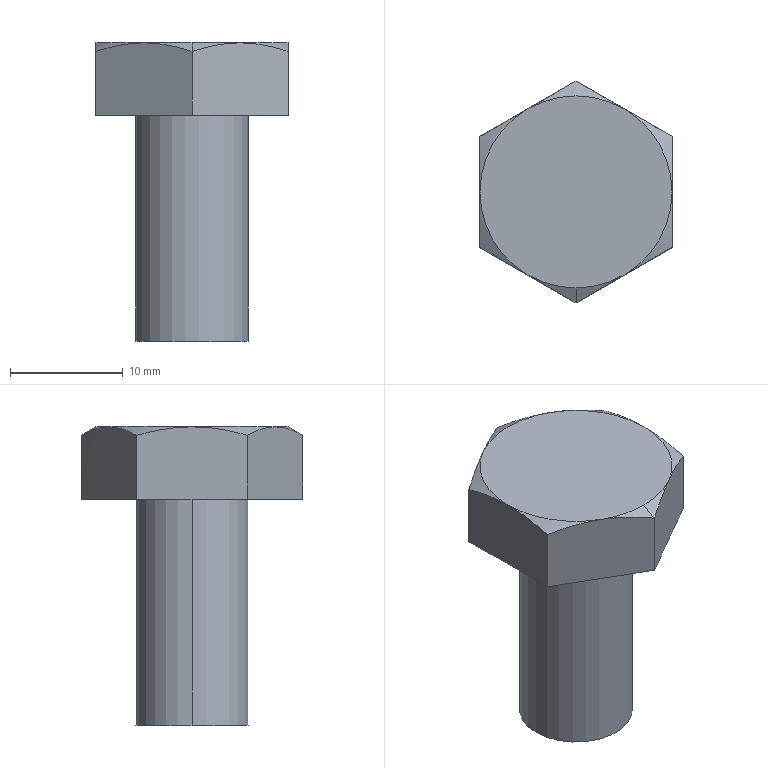Part | SolidWorks | features ICE 1, MBimport 1 | 1 solid | 18 faces | box 17 x 19.63 x 26.4 mm | volume 3167 mm3 | plane 9 | cone 7 | cylinder 2 | commonest cylinder face diameters 10 x2
STEP:
#1=CARTESIAN_POINT('',(-5.,0.,-10.));
#2=VERTEX_POINT('',#1);
#3=CARTESIAN_POINT('',(5.,0.,-10.));
#4=VERTEX_POINT('',#3);
#5=CARTESIAN_POINT('',(0.,0.,-10.));
#6=DIRECTION('',(0.,0.,-1.));
#7=DIRECTION('',(-1.,0.,0.));
#8=AXIS2_PLACEMENT_3D('',#5,#6,#7);
#9=CIRCLE('',#8,5.);
#10=EDGE_CURVE('',#2,#4,#9,.T.);
#11=ORIENTED_EDGE('',*,*,#10,.F.);
#12=CARTESIAN_POINT('',(-5.,0.,10.));
#13=VERTEX_POINT('',#12);
#14=CARTESIAN_POINT('',(-5.,0.,0.));
#15=DIRECTION('',(0.,0.,1.));
#16=VECTOR('',#15,1000.);
#17=LINE('',#14,#16);
#18=EDGE_CURVE('',#2,#13,#17,.T.);
#19=ORIENTED_EDGE('',*,*,#18,.T.);
#20=CARTESIAN_POINT('',(5.,0.,10.));
#21=VERTEX_POINT('',#20);
#22=CARTESIAN_POINT('',(0.,0.,10.));
#23=DIRECTION('',(0.,0.,1.));
#24=DIRECTION('',(-1.,0.,0.));
#25=AXIS2_PLACEMENT_3D('',#22,#23,#24);
#26=CIRCLE('',#25,5.);
#27=EDGE_CURVE('',#21,#13,#26,.T.);
#28=ORIENTED_EDGE('',*,*,#27,.F.);
#29=CARTESIAN_POINT('',(5.,0.,0.));
#30=DIRECTION('',(0.,0.,1.));
#31=VECTOR('',#30,1000.);
#32=LINE('',#29,#31);
#33=EDGE_CURVE('',#4,#21,#32,.T.);
#34=ORIENTED_EDGE('',*,*,#33,.F.);
#35=EDGE_LOOP('',(#11,#19,#28,#34));
#36=FACE_OUTER_BOUND('',#35,.T.);
#37=CARTESIAN_POINT('',(0.,0.,0.));
#38=DIRECTION('',(0.,0.,1.));
#39=DIRECTION('',(1.,0.,0.));
#40=AXIS2_PLACEMENT_3D('',#37,#38,#39);
#41=CYLINDRICAL_SURFACE('',#40,5.);
#42=ADVANCED_FACE('',(#36),#41,.T.);
#43=CARTESIAN_POINT('',(0.,-8.5,16.4));
#44=VERTEX_POINT('',#43);
#45=CARTESIAN_POINT('',(4.25,-7.361,16.4));
#46=VERTEX_POINT('',#45);
#47=CARTESIAN_POINT('',(0.,0.,16.4));
#48=DIRECTION('',(0.,0.,1.));
#49=DIRECTION('',(-0.5,-0.866,0.));
#50=AXIS2_PLACEMENT_3D('',#47,#48,#49);
#51=CIRCLE('',#50,8.5);
#52=EDGE_CURVE('',#44,#46,#51,.T.);
#53=ORIENTED_EDGE('',*,*,#52,.F.);
#54=CARTESIAN_POINT('',(0.,-9.815,15.641));
#55=VERTEX_POINT('',#54);
#56=CARTESIAN_POINT('',(0.,-9.157,16.02));
#57=DIRECTION('',(0.,-0.866,-0.5));
#58=VECTOR('',#57,1000.);
#59=LINE('',#56,#58);
#60=EDGE_CURVE('',#44,#55,#59,.T.);
#61=ORIENTED_EDGE('',*,*,#60,.T.);
#62=CARTESIAN_POINT('',(0.,-9.815,15.641));
#63=CARTESIAN_POINT('',(0.3728,-9.6,15.765));
#64=CARTESIAN_POINT('',(0.7368,-9.389,15.874));
#65=CARTESIAN_POINT('',(1.275,-9.078,16.016));
#66=CARTESIAN_POINT('',(1.454,-8.975,16.059));
#67=CARTESIAN_POINT('',(1.809,-8.771,16.138));
#68=CARTESIAN_POINT('',(1.987,-8.668,16.175));
#69=CARTESIAN_POINT('',(2.514,-8.364,16.27));
#70=CARTESIAN_POINT('',(2.858,-8.165,16.318));
#71=CARTESIAN_POINT('',(3.557,-7.762,16.384));
#72=CARTESIAN_POINT('',(3.902,-7.562,16.4));
#73=CARTESIAN_POINT('',(4.25,-7.361,16.4));
#74=B_SPLINE_CURVE_WITH_KNOTS('',3,(#62,#63,#64,#65,#66,#67,#68,#69,#70,#71,#72,#73),.UNSPECIFIED.,.F.,.F.,(4,2,2,2,2,4),(0.,0.25,0.375,0.5,0.75,1.),.UNSPECIFIED.);
#75=EDGE_CURVE('',#55,#46,#74,.T.);
#76=ORIENTED_EDGE('',*,*,#75,.T.);
#77=EDGE_LOOP('',(#53,#61,#76));
#78=FACE_OUTER_BOUND('',#77,.T.);
#79=CARTESIAN_POINT('',(0.,0.,16.02));
#80=DIRECTION('',(0.,0.,-1.));
#81=DIRECTION('',(0.,-1.,0.));
#82=AXIS2_PLACEMENT_3D('',#79,#80,#81);
#83=CONICAL_SURFACE('',#82,9.157,1.047);
#84=ADVANCED_FACE('',(#78),#83,.T.);
#85=CARTESIAN_POINT('',(-8.5,4.907,10.));
#86=VERTEX_POINT('',#85);
#87=CARTESIAN_POINT('',(-8.5,4.907,15.641));
#88=VERTEX_POINT('',#87);
#89=CARTESIAN_POINT('',(-8.5,4.907,10.));
#90=DIRECTION('',(0.,0.,1.));
#91=VECTOR('',#90,1000.);
#92=LINE('',#89,#91);
#93=EDGE_CURVE('',#86,#88,#92,.T.);
#94=ORIENTED_EDGE('',*,*,#93,.F.);
#95=CARTESIAN_POINT('',(-8.5,-4.907,10.));
#96=VERTEX_POINT('',#95);
#97=CARTESIAN_POINT('',(-8.5,4.907,10.));
#98=DIRECTION('',(0.,-1.,0.));
#99=VECTOR('',#98,1000.);
#100=LINE('',#97,#99);
#101=EDGE_CURVE('',#86,#96,#100,.T.);
#102=ORIENTED_EDGE('',*,*,#101,.T.);
#103=CARTESIAN_POINT('',(-8.5,-4.907,15.641));
#104=VERTEX_POINT('',#103);
#105=CARTESIAN_POINT('',(-8.5,-4.907,10.));
#106=DIRECTION('',(0.,0.,1.));
#107=VECTOR('',#106,1000.);
#108=LINE('',#105,#107);
#109=EDGE_CURVE('',#96,#104,#108,.T.);
#110=ORIENTED_EDGE('',*,*,#109,.T.);
#111=CARTESIAN_POINT('',(-8.5,0.,16.4));
#112=VERTEX_POINT('',#111);
#113=CARTESIAN_POINT('',(-8.5,0.,16.4));
#114=CARTESIAN_POINT('',(-8.5,-0.201,16.4));
#115=CARTESIAN_POINT('',(-8.5,-0.4012,16.396));
#116=CARTESIAN_POINT('',(-8.5,-0.8019,16.38));
#117=CARTESIAN_POINT('',(-8.5,-1.004,16.367));
#118=CARTESIAN_POINT('',(-8.5,-1.405,16.335));
#119=CARTESIAN_POINT('',(-8.5,-1.605,16.315));
#120=CARTESIAN_POINT('',(-8.5,-2.007,16.266));
#121=CARTESIAN_POINT('',(-8.5,-2.207,16.239));
#122=CARTESIAN_POINT('',(-8.5,-3.227,16.078));
#123=CARTESIAN_POINT('',(-8.5,-4.047,15.889));
#124=CARTESIAN_POINT('',(-8.5,-4.907,15.641));
#125=B_SPLINE_CURVE_WITH_KNOTS('',3,(#113,#114,#115,#116,#117,#118,#119,#120,#121,#122,#123,#124),.UNSPECIFIED.,.F.,.F.,(4,2,2,2,2,4),(0.,0.125,0.25,0.375,0.5,1.),.UNSPECIFIED.);
#126=EDGE_CURVE('',#112,#104,#125,.T.);
#127=ORIENTED_EDGE('',*,*,#126,.F.);
#128=CARTESIAN_POINT('',(-8.5,4.907,15.641));
#129=CARTESIAN_POINT('',(-8.5,4.477,15.765));
#130=CARTESIAN_POINT('',(-8.5,4.057,15.874));
#131=CARTESIAN_POINT('',(-8.5,3.435,16.016));
#132=CARTESIAN_POINT('',(-8.5,3.229,16.059));
#133=CARTESIAN_POINT('',(-8.5,2.819,16.138));
#134=CARTESIAN_POINT('',(-8.5,2.613,16.175));
#135=CARTESIAN_POINT('',(-8.5,2.005,16.27));
#136=CARTESIAN_POINT('',(-8.5,1.607,16.318));
#137=CARTESIAN_POINT('',(-8.5,0.8006,16.384));
#138=CARTESIAN_POINT('',(-8.5,0.402,16.4));
#139=CARTESIAN_POINT('',(-8.5,0.,16.4));
#140=B_SPLINE_CURVE_WITH_KNOTS('',3,(#128,#129,#130,#131,#132,#133,#134,#135,#136,#137,#138,#139),.UNSPECIFIED.,.F.,.F.,(4,2,2,2,2,4),(0.,0.25,0.375,0.5,0.75,1.),.UNSPECIFIED.);
#141=EDGE_CURVE('',#88,#112,#140,.T.);
#142=ORIENTED_EDGE('',*,*,#141,.F.);
#143=EDGE_LOOP('',(#94,#102,#110,#127,#142));
#144=FACE_OUTER_BOUND('',#143,.T.);
#145=CARTESIAN_POINT('',(-8.5,4.907,10.));
#146=DIRECTION('',(-1.,0.,0.));
#147=DIRECTION('',(0.,0.,1.));
#148=AXIS2_PLACEMENT_3D('',#145,#146,#147);
#149=PLANE('',#148);
#150=ADVANCED_FACE('',(#144),#149,.T.);
#151=ORIENTED_EDGE('',*,*,#109,.F.);
#152=CARTESIAN_POINT('',(0.,-9.815,10.));
#153=VERTEX_POINT('',#152);
#154=CARTESIAN_POINT('',(-8.5,-4.907,10.));
#155=DIRECTION('',(0.866,-0.5,0.));
#156=VECTOR('',#155,1000.);
#157=LINE('',#154,#156);
#158=EDGE_CURVE('',#96,#153,#157,.T.);
#159=ORIENTED_EDGE('',*,*,#158,.T.);
#160=CARTESIAN_POINT('',(0.,-9.815,10.));
#161=DIRECTION('',(0.,0.,1.));
#162=VECTOR('',#161,1000.);
#163=LINE('',#160,#162);
#164=EDGE_CURVE('',#153,#55,#163,.T.);
#165=ORIENTED_EDGE('',*,*,#164,.T.);
#166=CARTESIAN_POINT('',(-4.25,-7.361,16.4));
#167=VERTEX_POINT('',#166);
#168=CARTESIAN_POINT('',(-4.25,-7.361,16.4));
#169=CARTESIAN_POINT('',(-4.076,-7.462,16.4));
#170=CARTESIAN_POINT('',(-3.903,-7.562,16.396));
#171=CARTESIAN_POINT('',(-3.556,-7.762,16.38));
#172=CARTESIAN_POINT('',(-3.381,-7.863,16.367));
#173=CARTESIAN_POINT('',(-3.034,-8.064,16.335));
#174=CARTESIAN_POINT('',(-2.86,-8.164,16.315));
#175=CARTESIAN_POINT('',(-2.512,-8.365,16.266));
#176=CARTESIAN_POINT('',(-2.339,-8.465,16.239));
#177=CARTESIAN_POINT('',(-1.455,-8.975,16.078));
#178=CARTESIAN_POINT('',(-0.7455,-9.385,15.889));
#179=CARTESIAN_POINT('',(0.,-9.815,15.641));
#180=B_SPLINE_CURVE_WITH_KNOTS('',3,(#168,#169,#170,#171,#172,#173,#174,#175,#176,#177,#178,#179),.UNSPECIFIED.,.F.,.F.,(4,2,2,2,2,4),(0.,0.125,0.25,0.375,0.5,1.),.UNSPECIFIED.);
#181=EDGE_CURVE('',#167,#55,#180,.T.);
#182=ORIENTED_EDGE('',*,*,#181,.F.);
#183=CARTESIAN_POINT('',(-8.5,-4.907,15.641));
#184=CARTESIAN_POINT('',(-8.127,-5.123,15.765));
#185=CARTESIAN_POINT('',(-7.763,-5.333,15.874));
#186=CARTESIAN_POINT('',(-7.224,-5.644,16.016));
#187=CARTESIAN_POINT('',(-7.046,-5.747,16.059));
#188=CARTESIAN_POINT('',(-6.691,-5.952,16.138));
#189=CARTESIAN_POINT('',(-6.513,-6.054,16.175));
#190=CARTESIAN_POINT('',(-5.986,-6.359,16.27));
#191=CARTESIAN_POINT('',(-5.642,-6.558,16.318));
#192=CARTESIAN_POINT('',(-4.943,-6.961,16.384));
#193=CARTESIAN_POINT('',(-4.598,-7.16,16.4));
#194=CARTESIAN_POINT('',(-4.25,-7.361,16.4));
#195=B_SPLINE_CURVE_WITH_KNOTS('',3,(#183,#184,#185,#186,#187,#188,#189,#190,#191,#192,#193,#194),.UNSPECIFIED.,.F.,.F.,(4,2,2,2,2,4),(0.,0.25,0.375,0.5,0.75,1.),.UNSPECIFIED.);
#196=EDGE_CURVE('',#104,#167,#195,.T.);
#197=ORIENTED_EDGE('',*,*,#196,.F.);
#198=EDGE_LOOP('',(#151,#159,#165,#182,#197));
#199=FACE_OUTER_BOUND('',#198,.T.);
#200=CARTESIAN_POINT('',(-8.5,-4.907,10.));
#201=DIRECTION('',(-0.5,-0.866,0.));
#202=DIRECTION('',(-0.866,0.5,0.));
#203=AXIS2_PLACEMENT_3D('',#200,#201,#202);
#204=PLANE('',#203);
#205=ADVANCED_FACE('',(#199),#204,.T.);
#206=ORIENTED_EDGE('',*,*,#164,.F.);
#207=CARTESIAN_POINT('',(8.5,-4.907,10.));
#208=VERTEX_POINT('',#207);
#209=CARTESIAN_POINT('',(0.,-9.815,10.));
#210=DIRECTION('',(0.866,0.5,0.));
#211=VECTOR('',#210,1000.);
#212=LINE('',#209,#211);
#213=EDGE_CURVE('',#153,#208,#212,.T.);
#214=ORIENTED_EDGE('',*,*,#213,.T.);
#215=CARTESIAN_POINT('',(8.5,-4.907,15.641));
#216=VERTEX_POINT('',#215);
#217=CARTESIAN_POINT('',(8.5,-4.907,10.));
#218=DIRECTION('',(0.,0.,1.));
#219=VECTOR('',#218,1000.);
#220=LINE('',#217,#219);
#221=EDGE_CURVE('',#208,#216,#220,.T.);
#222=ORIENTED_EDGE('',*,*,#221,.T.);
#223=CARTESIAN_POINT('',(4.25,-7.361,16.4));
#224=CARTESIAN_POINT('',(4.424,-7.261,16.4));
#225=CARTESIAN_POINT('',(4.597,-7.161,16.396));
#226=CARTESIAN_POINT('',(4.944,-6.96,16.38));
#227=CARTESIAN_POINT('',(5.119,-6.859,16.367));
#228=CARTESIAN_POINT('',(5.466,-6.659,16.335));
#229=CARTESIAN_POINT('',(5.64,-6.559,16.315));
#230=CARTESIAN_POINT('',(5.988,-6.358,16.266));
#231=CARTESIAN_POINT('',(6.161,-6.258,16.239));
#232=CARTESIAN_POINT('',(7.045,-5.748,16.078));
#233=CARTESIAN_POINT('',(7.754,-5.338,15.889));
#234=CARTESIAN_POINT('',(8.5,-4.907,15.641));
#235=B_SPLINE_CURVE_WITH_KNOTS('',3,(#223,#224,#225,#226,#227,#228,#229,#230,#231,#232,#233,#234),.UNSPECIFIED.,.F.,.F.,(4,2,2,2,2,4),(0.,0.125,0.25,0.375,0.5,1.),.UNSPECIFIED.);
#236=EDGE_CURVE('',#46,#216,#235,.T.);
#237=ORIENTED_EDGE('',*,*,#236,.F.);
#238=ORIENTED_EDGE('',*,*,#75,.F.);
#239=EDGE_LOOP('',(#206,#214,#222,#237,#238));
#240=FACE_OUTER_BOUND('',#239,.T.);
#241=CARTESIAN_POINT('',(0.,-9.815,10.));
#242=DIRECTION('',(0.5,-0.866,0.));
#243=DIRECTION('',(0.,0.,-1.));
#244=AXIS2_PLACEMENT_3D('',#241,#242,#243);
#245=PLANE('',#244);
#246=ADVANCED_FACE('',(#240),#245,.T.);
#247=ORIENTED_EDGE('',*,*,#221,.F.);
#248=CARTESIAN_POINT('',(8.5,4.907,10.));
#249=VERTEX_POINT('',#248);
#250=CARTESIAN_POINT('',(8.5,-4.907,10.));
#251=DIRECTION('',(0.,1.,0.));
#252=VECTOR('',#251,1000.);
#253=LINE('',#250,#252);
#254=EDGE_CURVE('',#208,#249,#253,.T.);
#255=ORIENTED_EDGE('',*,*,#254,.T.);
#256=CARTESIAN_POINT('',(8.5,4.907,15.641));
#257=VERTEX_POINT('',#256);
#258=CARTESIAN_POINT('',(8.5,4.907,10.));
#259=DIRECTION('',(0.,0.,1.));
#260=VECTOR('',#259,1000.);
#261=LINE('',#258,#260);
#262=EDGE_CURVE('',#249,#257,#261,.T.);
#263=ORIENTED_EDGE('',*,*,#262,.T.);
#264=CARTESIAN_POINT('',(8.5,0.,16.4));
#265=VERTEX_POINT('',#264);
#266=CARTESIAN_POINT('',(8.5,0.,16.4));
#267=CARTESIAN_POINT('',(8.5,0.201,16.4));
#268=CARTESIAN_POINT('',(8.5,0.4012,16.396));
#269=CARTESIAN_POINT('',(8.5,0.8019,16.38));
#270=CARTESIAN_POINT('',(8.5,1.004,16.367));
#271=CARTESIAN_POINT('',(8.5,1.405,16.335));
#272=CARTESIAN_POINT('',(8.5,1.605,16.315));
#273=CARTESIAN_POINT('',(8.5,2.007,16.266));
#274=CARTESIAN_POINT('',(8.5,2.207,16.239));
#275=CARTESIAN_POINT('',(8.5,3.227,16.078));
#276=CARTESIAN_POINT('',(8.5,4.047,15.889));
#277=CARTESIAN_POINT('',(8.5,4.907,15.641));
#278=B_SPLINE_CURVE_WITH_KNOTS('',3,(#266,#267,#268,#269,#270,#271,#272,#273,#274,#275,#276,#277),.UNSPECIFIED.,.F.,.F.,(4,2,2,2,2,4),(0.,0.125,0.25,0.375,0.5,1.),.UNSPECIFIED.);
#279=EDGE_CURVE('',#265,#257,#278,.T.);
#280=ORIENTED_EDGE('',*,*,#279,.F.);
#281=CARTESIAN_POINT('',(8.5,-4.907,15.641));
#282=CARTESIAN_POINT('',(8.5,-4.477,15.765));
#283=CARTESIAN_POINT('',(8.5,-4.057,15.874));
#284=CARTESIAN_POINT('',(8.5,-3.435,16.016));
#285=CARTESIAN_POINT('',(8.5,-3.229,16.059));
#286=CARTESIAN_POINT('',(8.5,-2.819,16.138));
#287=CARTESIAN_POINT('',(8.5,-2.613,16.175));
#288=CARTESIAN_POINT('',(8.5,-2.005,16.27));
#289=CARTESIAN_POINT('',(8.5,-1.607,16.318));
#290=CARTESIAN_POINT('',(8.5,-0.8006,16.384));
#291=CARTESIAN_POINT('',(8.5,-0.402,16.4));
#292=CARTESIAN_POINT('',(8.5,0.,16.4));
#293=B_SPLINE_CURVE_WITH_KNOTS('',3,(#281,#282,#283,#284,#285,#286,#287,#288,#289,#290,#291,#292),.UNSPECIFIED.,.F.,.F.,(4,2,2,2,2,4),(0.,0.25,0.375,0.5,0.75,1.),.UNSPECIFIED.);
#294=EDGE_CURVE('',#216,#265,#293,.T.);
#295=ORIENTED_EDGE('',*,*,#294,.F.);
#296=EDGE_LOOP('',(#247,#255,#263,#280,#295));
#297=FACE_OUTER_BOUND('',#296,.T.);
#298=CARTESIAN_POINT('',(8.5,-4.907,10.));
#299=DIRECTION('',(1.,0.,0.));
#300=DIRECTION('',(0.,1.,0.));
#301=AXIS2_PLACEMENT_3D('',#298,#299,#300);
#302=PLANE('',#301);
#303=ADVANCED_FACE('',(#297),#302,.T.);
#304=ORIENTED_EDGE('',*,*,#262,.F.);
#305=CARTESIAN_POINT('',(0.,9.815,10.));
#306=VERTEX_POINT('',#305);
#307=CARTESIAN_POINT('',(8.5,4.907,10.));
#308=DIRECTION('',(-0.866,0.5,0.));
#309=VECTOR('',#308,1000.);
#310=LINE('',#307,#309);
#311=EDGE_CURVE('',#249,#306,#310,.T.);
#312=ORIENTED_EDGE('',*,*,#311,.T.);
#313=CARTESIAN_POINT('',(0.,9.815,15.641));
#314=VERTEX_POINT('',#313);
#315=CARTESIAN_POINT('',(0.,9.815,10.));
#316=DIRECTION('',(0.,0.,1.));
#317=VECTOR('',#316,1000.);
#318=LINE('',#315,#317);
#319=EDGE_CURVE('',#306,#314,#318,.T.);
#320=ORIENTED_EDGE('',*,*,#319,.T.);
#321=CARTESIAN_POINT('',(4.25,7.361,16.4));
#322=VERTEX_POINT('',#321);
#323=CARTESIAN_POINT('',(4.25,7.361,16.4));
#324=CARTESIAN_POINT('',(4.076,7.462,16.4));
#325=CARTESIAN_POINT('',(3.903,7.562,16.396));
#326=CARTESIAN_POINT('',(3.556,7.762,16.38));
#327=CARTESIAN_POINT('',(3.381,7.863,16.367));
#328=CARTESIAN_POINT('',(3.034,8.064,16.335));
#329=CARTESIAN_POINT('',(2.86,8.164,16.315));
#330=CARTESIAN_POINT('',(2.512,8.365,16.266));
#331=CARTESIAN_POINT('',(2.339,8.465,16.239));
#332=CARTESIAN_POINT('',(1.455,8.975,16.078));
#333=CARTESIAN_POINT('',(0.7455,9.385,15.889));
#334=CARTESIAN_POINT('',(0.,9.815,15.641));
#335=B_SPLINE_CURVE_WITH_KNOTS('',3,(#323,#324,#325,#326,#327,#328,#329,#330,#331,#332,#333,#334),.UNSPECIFIED.,.F.,.F.,(4,2,2,2,2,4),(0.,0.125,0.25,0.375,0.5,1.),.UNSPECIFIED.);
#336=EDGE_CURVE('',#322,#314,#335,.T.);
#337=ORIENTED_EDGE('',*,*,#336,.F.);
#338=CARTESIAN_POINT('',(8.5,4.907,15.641));
#339=CARTESIAN_POINT('',(8.127,5.123,15.765));
#340=CARTESIAN_POINT('',(7.763,5.333,15.874));
#341=CARTESIAN_POINT('',(7.224,5.644,16.016));
#342=CARTESIAN_POINT('',(7.046,5.747,16.059));
#343=CARTESIAN_POINT('',(6.691,5.952,16.138));
#344=CARTESIAN_POINT('',(6.513,6.054,16.175));
#345=CARTESIAN_POINT('',(5.986,6.359,16.27));
#346=CARTESIAN_POINT('',(5.642,6.558,16.318));
#347=CARTESIAN_POINT('',(4.943,6.961,16.384));
#348=CARTESIAN_POINT('',(4.598,7.16,16.4));
#349=CARTESIAN_POINT('',(4.25,7.361,16.4));
#350=B_SPLINE_CURVE_WITH_KNOTS('',3,(#338,#339,#340,#341,#342,#343,#344,#345,#346,#347,#348,#349),.UNSPECIFIED.,.F.,.F.,(4,2,2,2,2,4),(0.,0.25,0.375,0.5,0.75,1.),.UNSPECIFIED.);
#351=EDGE_CURVE('',#257,#322,#350,.T.);
#352=ORIENTED_EDGE('',*,*,#351,.F.);
#353=EDGE_LOOP('',(#304,#312,#320,#337,#352));
#354=FACE_OUTER_BOUND('',#353,.T.);
#355=CARTESIAN_POINT('',(8.5,4.907,10.));
#356=DIRECTION('',(0.5,0.866,0.));
#357=DIRECTION('',(0.,0.,-1.));
#358=AXIS2_PLACEMENT_3D('',#355,#356,#357);
#359=PLANE('',#358);
#360=ADVANCED_FACE('',(#354),#359,.T.);
#361=ORIENTED_EDGE('',*,*,#60,.F.);
#362=CARTESIAN_POINT('',(0.,0.,16.4));
#363=DIRECTION('',(0.,0.,1.));
#364=DIRECTION('',(-0.5,-0.866,0.));
#365=AXIS2_PLACEMENT_3D('',#362,#363,#364);
#366=CIRCLE('',#365,8.5);
#367=EDGE_CURVE('',#167,#44,#366,.T.);
#368=ORIENTED_EDGE('',*,*,#367,.F.);
#369=ORIENTED_EDGE('',*,*,#181,.T.);
#370=EDGE_LOOP('',(#361,#368,#369));
#371=FACE_OUTER_BOUND('',#370,.T.);
#372=CARTESIAN_POINT('',(0.,0.,16.02));
#373=DIRECTION('',(0.,0.,-1.));
#374=DIRECTION('',(0.,-1.,0.));
#375=AXIS2_PLACEMENT_3D('',#372,#373,#374);
#376=CONICAL_SURFACE('',#375,9.157,1.047);
#377=ADVANCED_FACE('',(#371),#376,.T.);
#378=ORIENTED_EDGE('',*,*,#126,.T.);
#379=ORIENTED_EDGE('',*,*,#196,.T.);
#380=CARTESIAN_POINT('',(0.,0.,16.4));
#381=DIRECTION('',(0.,0.,1.));
#382=DIRECTION('',(-1.,0.,0.));
#383=AXIS2_PLACEMENT_3D('',#380,#381,#382);
#384=CIRCLE('',#383,8.5);
#385=EDGE_CURVE('',#112,#167,#384,.T.);
#386=ORIENTED_EDGE('',*,*,#385,.F.);
#387=EDGE_LOOP('',(#378,#379,#386));
#388=FACE_OUTER_BOUND('',#387,.T.);
#389=CARTESIAN_POINT('',(0.,0.,16.02));
#390=DIRECTION('',(0.,0.,-1.));
#391=DIRECTION('',(0.,-1.,0.));
#392=AXIS2_PLACEMENT_3D('',#389,#390,#391);
#393=CONICAL_SURFACE('',#392,9.157,1.047);
#394=ADVANCED_FACE('',(#388),#393,.T.);
#395=CARTESIAN_POINT('',(-4.25,7.361,16.4));
#396=VERTEX_POINT('',#395);
#397=CARTESIAN_POINT('',(-4.25,7.361,16.4));
#398=CARTESIAN_POINT('',(-4.424,7.261,16.4));
#399=CARTESIAN_POINT('',(-4.597,7.161,16.396));
#400=CARTESIAN_POINT('',(-4.944,6.96,16.38));
#401=CARTESIAN_POINT('',(-5.119,6.859,16.367));
#402=CARTESIAN_POINT('',(-5.466,6.659,16.335));
#403=CARTESIAN_POINT('',(-5.64,6.559,16.315));
#404=CARTESIAN_POINT('',(-5.988,6.358,16.266));
#405=CARTESIAN_POINT('',(-6.161,6.258,16.239));
#406=CARTESIAN_POINT('',(-7.045,5.748,16.078));
#407=CARTESIAN_POINT('',(-7.754,5.338,15.889));
#408=CARTESIAN_POINT('',(-8.5,4.907,15.641));
#409=B_SPLINE_CURVE_WITH_KNOTS('',3,(#397,#398,#399,#400,#401,#402,#403,#404,#405,#406,#407,#408),.UNSPECIFIED.,.F.,.F.,(4,2,2,2,2,4),(0.,0.125,0.25,0.375,0.5,1.),.UNSPECIFIED.);
#410=EDGE_CURVE('',#396,#88,#409,.T.);
#411=ORIENTED_EDGE('',*,*,#410,.T.);
#412=ORIENTED_EDGE('',*,*,#141,.T.);
#413=CARTESIAN_POINT('',(0.,0.,16.4));
#414=DIRECTION('',(0.,0.,1.));
#415=DIRECTION('',(-0.5,0.866,0.));
#416=AXIS2_PLACEMENT_3D('',#413,#414,#415);
#417=CIRCLE('',#416,8.5);
#418=EDGE_CURVE('',#396,#112,#417,.T.);
#419=ORIENTED_EDGE('',*,*,#418,.F.);
#420=EDGE_LOOP('',(#411,#412,#419));
#421=FACE_OUTER_BOUND('',#420,.T.);
#422=CARTESIAN_POINT('',(0.,0.,16.02));
#423=DIRECTION('',(0.,0.,-1.));
#424=DIRECTION('',(0.,-1.,0.));
#425=AXIS2_PLACEMENT_3D('',#422,#423,#424);
#426=CONICAL_SURFACE('',#425,9.157,1.047);
#427=ADVANCED_FACE('',(#421),#426,.T.);
#428=ORIENTED_EDGE('',*,*,#236,.T.);
#429=ORIENTED_EDGE('',*,*,#294,.T.);
#430=CARTESIAN_POINT('',(0.,0.,16.4));
#431=DIRECTION('',(0.,0.,1.));
#432=DIRECTION('',(0.5,-0.866,0.));
#433=AXIS2_PLACEMENT_3D('',#430,#431,#432);
#434=CIRCLE('',#433,8.5);
#435=EDGE_CURVE('',#46,#265,#434,.T.);
#436=ORIENTED_EDGE('',*,*,#435,.F.);
#437=EDGE_LOOP('',(#428,#429,#436));
#438=FACE_OUTER_BOUND('',#437,.T.);
#439=CARTESIAN_POINT('',(0.,0.,16.02));
#440=DIRECTION('',(0.,0.,-1.));
#441=DIRECTION('',(0.,-1.,0.));
#442=AXIS2_PLACEMENT_3D('',#439,#440,#441);
#443=CONICAL_SURFACE('',#442,9.157,1.047);
#444=ADVANCED_FACE('',(#438),#443,.T.);
#445=ORIENTED_EDGE('',*,*,#279,.T.);
#446=ORIENTED_EDGE('',*,*,#351,.T.);
#447=CARTESIAN_POINT('',(0.,0.,16.4));
#448=DIRECTION('',(0.,0.,1.));
#449=DIRECTION('',(1.,0.,0.));
#450=AXIS2_PLACEMENT_3D('',#447,#448,#449);
#451=CIRCLE('',#450,8.5);
#452=EDGE_CURVE('',#265,#322,#451,.T.);
#453=ORIENTED_EDGE('',*,*,#452,.F.);
#454=EDGE_LOOP('',(#445,#446,#453));
#455=FACE_OUTER_BOUND('',#454,.T.);
#456=CARTESIAN_POINT('',(0.,0.,16.02));
#457=DIRECTION('',(0.,0.,-1.));
#458=DIRECTION('',(0.,-1.,0.));
#459=AXIS2_PLACEMENT_3D('',#456,#457,#458);
#460=CONICAL_SURFACE('',#459,9.157,1.047);
#461=ADVANCED_FACE('',(#455),#460,.T.);
#462=ORIENTED_EDGE('',*,*,#435,.T.);
#463=ORIENTED_EDGE('',*,*,#452,.T.);
#464=CARTESIAN_POINT('',(0.,0.,16.4));
#465=DIRECTION('',(0.,0.,1.));
#466=DIRECTION('',(0.5,0.866,0.));
#467=AXIS2_PLACEMENT_3D('',#464,#465,#466);
#468=CIRCLE('',#467,8.5);
#469=EDGE_CURVE('',#322,#396,#468,.T.);
#470=ORIENTED_EDGE('',*,*,#469,.T.);
#471=ORIENTED_EDGE('',*,*,#418,.T.);
#472=ORIENTED_EDGE('',*,*,#385,.T.);
#473=ORIENTED_EDGE('',*,*,#367,.T.);
#474=ORIENTED_EDGE('',*,*,#52,.T.);
#475=EDGE_LOOP('',(#462,#463,#470,#471,#472,#473,#474));
#476=FACE_OUTER_BOUND('',#475,.T.);
#477=CARTESIAN_POINT('',(0.,0.,16.4));
#478=DIRECTION('',(0.,0.,1.));
#479=DIRECTION('',(1.,0.,0.));
#480=AXIS2_PLACEMENT_3D('',#477,#478,#479);
#481=PLANE('',#480);
#482=ADVANCED_FACE('',(#476),#481,.T.);
#483=ORIENTED_EDGE('',*,*,#336,.T.);
#484=CARTESIAN_POINT('',(0.,9.815,15.641));
#485=CARTESIAN_POINT('',(-0.3728,9.6,15.765));
#486=CARTESIAN_POINT('',(-0.7368,9.389,15.874));
#487=CARTESIAN_POINT('',(-1.275,9.078,16.016));
#488=CARTESIAN_POINT('',(-1.454,8.975,16.059));
#489=CARTESIAN_POINT('',(-1.809,8.771,16.138));
#490=CARTESIAN_POINT('',(-1.987,8.668,16.175));
#491=CARTESIAN_POINT('',(-2.514,8.364,16.27));
#492=CARTESIAN_POINT('',(-2.858,8.165,16.318));
#493=CARTESIAN_POINT('',(-3.557,7.762,16.384));
#494=CARTESIAN_POINT('',(-3.902,7.562,16.4));
#495=CARTESIAN_POINT('',(-4.25,7.361,16.4));
#496=B_SPLINE_CURVE_WITH_KNOTS('',3,(#484,#485,#486,#487,#488,#489,#490,#491,#492,#493,#494,#495),.UNSPECIFIED.,.F.,.F.,(4,2,2,2,2,4),(0.,0.25,0.375,0.5,0.75,1.),.UNSPECIFIED.);
#497=EDGE_CURVE('',#314,#396,#496,.T.);
#498=ORIENTED_EDGE('',*,*,#497,.T.);
#499=ORIENTED_EDGE('',*,*,#469,.F.);
#500=EDGE_LOOP('',(#483,#498,#499));
#501=FACE_OUTER_BOUND('',#500,.T.);
#502=CARTESIAN_POINT('',(0.,0.,16.02));
#503=DIRECTION('',(0.,0.,-1.));
#504=DIRECTION('',(0.,-1.,0.));
#505=AXIS2_PLACEMENT_3D('',#502,#503,#504);
#506=CONICAL_SURFACE('',#505,9.157,1.047);
#507=ADVANCED_FACE('',(#501),#506,.T.);
#508=ORIENTED_EDGE('',*,*,#319,.F.);
#509=CARTESIAN_POINT('',(0.,9.815,10.));
#510=DIRECTION('',(-0.866,-0.5,0.));
#511=VECTOR('',#510,1000.);
#512=LINE('',#509,#511);
#513=EDGE_CURVE('',#306,#86,#512,.T.);
#514=ORIENTED_EDGE('',*,*,#513,.T.);
#515=ORIENTED_EDGE('',*,*,#93,.T.);
#516=ORIENTED_EDGE('',*,*,#410,.F.);
#517=ORIENTED_EDGE('',*,*,#497,.F.);
#518=EDGE_LOOP('',(#508,#514,#515,#516,#517));
#519=FACE_OUTER_BOUND('',#518,.T.);
#520=CARTESIAN_POINT('',(0.,9.815,10.));
#521=DIRECTION('',(-0.5,0.866,0.));
#522=DIRECTION('',(0.,0.,1.));
#523=AXIS2_PLACEMENT_3D('',#520,#521,#522);
#524=PLANE('',#523);
#525=ADVANCED_FACE('',(#519),#524,.T.);
#526=ORIENTED_EDGE('',*,*,#27,.T.);
#527=CARTESIAN_POINT('',(0.,0.,10.));
#528=DIRECTION('',(0.,0.,1.));
#529=DIRECTION('',(-1.,0.,0.));
#530=AXIS2_PLACEMENT_3D('',#527,#528,#529);
#531=CIRCLE('',#530,5.);
#532=EDGE_CURVE('',#13,#21,#531,.T.);
#533=ORIENTED_EDGE('',*,*,#532,.T.);
#534=EDGE_LOOP('',(#526,#533));
#535=FACE_BOUND('',#534,.T.);
#536=ORIENTED_EDGE('',*,*,#311,.F.);
#537=ORIENTED_EDGE('',*,*,#254,.F.);
#538=ORIENTED_EDGE('',*,*,#213,.F.);
#539=ORIENTED_EDGE('',*,*,#158,.F.);
#540=ORIENTED_EDGE('',*,*,#101,.F.);
#541=ORIENTED_EDGE('',*,*,#513,.F.);
#542=EDGE_LOOP('',(#536,#537,#538,#539,#540,#541));
#543=FACE_OUTER_BOUND('',#542,.T.);
#544=CARTESIAN_POINT('',(0.,0.,10.));
#545=DIRECTION('',(0.,0.,1.));
#546=DIRECTION('',(1.,0.,0.));
#547=AXIS2_PLACEMENT_3D('',#544,#545,#546);
#548=PLANE('',#547);
#549=ADVANCED_FACE('',(#535,#543),#548,.F.);
#550=ORIENTED_EDGE('',*,*,#18,.F.);
#551=CARTESIAN_POINT('',(0.,0.,-10.));
#552=DIRECTION('',(0.,0.,-1.));
#553=DIRECTION('',(-1.,0.,0.));
#554=AXIS2_PLACEMENT_3D('',#551,#552,#553);
#555=CIRCLE('',#554,5.);
#556=EDGE_CURVE('',#4,#2,#555,.T.);
#557=ORIENTED_EDGE('',*,*,#556,.F.);
#558=ORIENTED_EDGE('',*,*,#33,.T.);
#559=ORIENTED_EDGE('',*,*,#532,.F.);
#560=EDGE_LOOP('',(#550,#557,#558,#559));
#561=FACE_OUTER_BOUND('',#560,.T.);
#562=CARTESIAN_POINT('',(0.,0.,0.));
#563=DIRECTION('',(0.,0.,1.));
#564=DIRECTION('',(1.,0.,0.));
#565=AXIS2_PLACEMENT_3D('',#562,#563,#564);
#566=CYLINDRICAL_SURFACE('',#565,5.);
#567=ADVANCED_FACE('',(#561),#566,.T.);
#568=ORIENTED_EDGE('',*,*,#556,.T.);
#569=ORIENTED_EDGE('',*,*,#10,.T.);
#570=EDGE_LOOP('',(#568,#569));
#571=FACE_OUTER_BOUND('',#570,.T.);
#572=CARTESIAN_POINT('',(0.,0.,-10.));
#573=DIRECTION('',(0.,0.,-1.));
#574=DIRECTION('',(-1.,0.,0.));
#575=AXIS2_PLACEMENT_3D('',#572,#573,#574);
#576=PLANE('',#575);
#577=ADVANCED_FACE('',(#571),#576,.T.);
#578=CLOSED_SHELL('',(#42,#84,#150,#205,#246,#303,#360,#377,#394,#427,#444,#461,#482,#507,#525,#549,#567,#577));
#579=MANIFOLD_SOLID_BREP('',#578);
#580=CARTESIAN_POINT('',(0.,0.,0.));
#581=DIRECTION('',(0.,0.,1.));
#582=DIRECTION('',(1.,0.,0.));
#583=AXIS2_PLACEMENT_3D('',#580,#581,#582);
#584=(LENGTH_UNIT()NAMED_UNIT(*)SI_UNIT(.MILLI.,.METRE.));
#585=UNCERTAINTY_MEASURE_WITH_UNIT(LENGTH_MEASURE(0.00001),#584,'','');
#586=(NAMED_UNIT(*)PLANE_ANGLE_UNIT()SI_UNIT($,.RADIAN.));
#587=(NAMED_UNIT(*)SI_UNIT($,.STERADIAN.)SOLID_ANGLE_UNIT());
#588=(GEOMETRIC_REPRESENTATION_CONTEXT(3)GLOBAL_UNCERTAINTY_ASSIGNED_CONTEXT((#585))GLOBAL_UNIT_ASSIGNED_CONTEXT((#584,#586,#587))REPRESENTATION_CONTEXT('',''));
#589=ADVANCED_BREP_SHAPE_REPRESENTATION('',(#579,#583),#588);